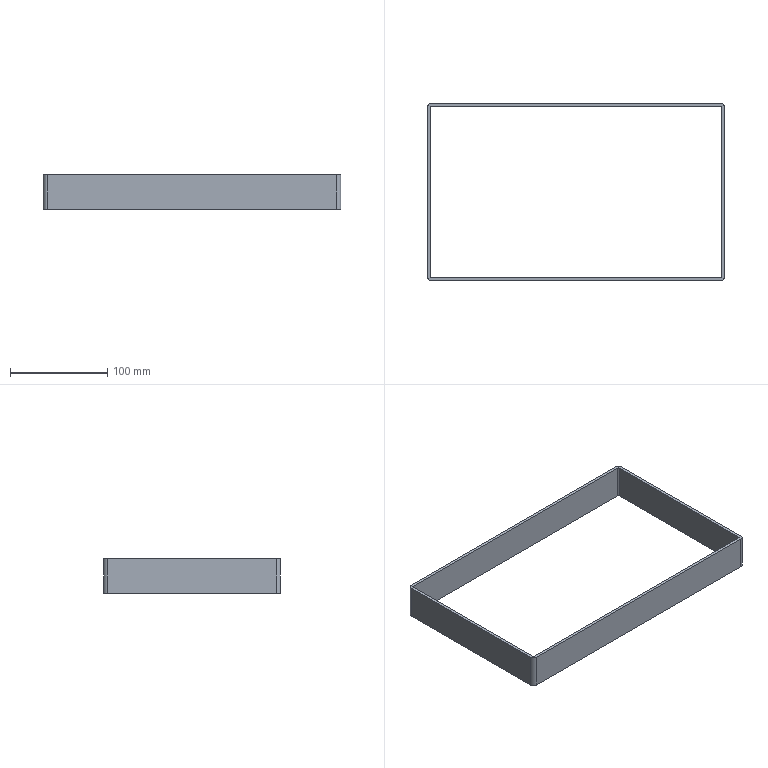Part | NX | features DATUM_CSYS 1, EXTRACT_DATUM_PLANE 1, EXTRUDE 1, SKETCH 1 | 1 solid | 18 faces | box 306 x 182 x 35 mm | volume 100769 mm3 | plane 10 | cylinder 8 | commonest cylinder face diameters 2 x4 8 x4
STEP:
#1=CARTESIAN_POINT('',(-150.,87.,0.));
#2=VERTEX_POINT('',#1);
#3=CARTESIAN_POINT('',(-150.,-87.,0.));
#4=VERTEX_POINT('',#3);
#5=CARTESIAN_POINT('',(-150.,87.,0.));
#6=DIRECTION('',(0.,-1.,0.));
#7=VECTOR('',#6,1000.);
#8=LINE('',#5,#7);
#9=EDGE_CURVE('',#2,#4,#8,.T.);
#10=ORIENTED_EDGE('',*,*,#9,.F.);
#11=CARTESIAN_POINT('',(-150.,87.,35.));
#12=VERTEX_POINT('',#11);
#13=CARTESIAN_POINT('',(-150.,87.,35.));
#14=DIRECTION('',(0.,0.,-1.));
#15=VECTOR('',#14,1000.);
#16=LINE('',#13,#15);
#17=EDGE_CURVE('',#12,#2,#16,.T.);
#18=ORIENTED_EDGE('',*,*,#17,.F.);
#19=CARTESIAN_POINT('',(-150.,-87.,35.));
#20=VERTEX_POINT('',#19);
#21=CARTESIAN_POINT('',(-150.,87.,35.));
#22=DIRECTION('',(0.,-1.,0.));
#23=VECTOR('',#22,1000.);
#24=LINE('',#21,#23);
#25=EDGE_CURVE('',#12,#20,#24,.T.);
#26=ORIENTED_EDGE('',*,*,#25,.T.);
#27=CARTESIAN_POINT('',(-150.,-87.,35.));
#28=DIRECTION('',(0.,0.,-1.));
#29=VECTOR('',#28,1000.);
#30=LINE('',#27,#29);
#31=EDGE_CURVE('',#20,#4,#30,.T.);
#32=ORIENTED_EDGE('',*,*,#31,.T.);
#33=EDGE_LOOP('',(#10,#18,#26,#32));
#34=FACE_BOUND('',#33,.T.);
#35=CARTESIAN_POINT('',(-150.,87.,35.));
#36=DIRECTION('',(1.,0.,0.));
#37=DIRECTION('',(0.,0.,-1.));
#38=AXIS2_PLACEMENT_3D('',#35,#36,#37);
#39=PLANE('',#38);
#40=ADVANCED_FACE('',(#34),#39,.T.);
#41=CARTESIAN_POINT('',(-149.,-88.,0.));
#42=VERTEX_POINT('',#41);
#43=CARTESIAN_POINT('',(-149.,-87.,0.));
#44=DIRECTION('',(0.,0.,1.));
#45=DIRECTION('',(-1.,0.,0.));
#46=AXIS2_PLACEMENT_3D('',#43,#44,#45);
#47=CIRCLE('',#46,1.);
#48=EDGE_CURVE('',#4,#42,#47,.T.);
#49=ORIENTED_EDGE('',*,*,#48,.F.);
#50=ORIENTED_EDGE('',*,*,#31,.F.);
#51=CARTESIAN_POINT('',(-149.,-88.,35.));
#52=VERTEX_POINT('',#51);
#53=CARTESIAN_POINT('',(-149.,-87.,35.));
#54=DIRECTION('',(0.,0.,1.));
#55=DIRECTION('',(-1.,0.,0.));
#56=AXIS2_PLACEMENT_3D('',#53,#54,#55);
#57=CIRCLE('',#56,1.);
#58=EDGE_CURVE('',#20,#52,#57,.T.);
#59=ORIENTED_EDGE('',*,*,#58,.T.);
#60=CARTESIAN_POINT('',(-149.,-88.,35.));
#61=DIRECTION('',(0.,0.,-1.));
#62=VECTOR('',#61,1000.);
#63=LINE('',#60,#62);
#64=EDGE_CURVE('',#52,#42,#63,.T.);
#65=ORIENTED_EDGE('',*,*,#64,.T.);
#66=EDGE_LOOP('',(#49,#50,#59,#65));
#67=FACE_BOUND('',#66,.T.);
#68=CARTESIAN_POINT('',(-149.,-87.,35.));
#69=DIRECTION('',(0.,0.,-1.));
#70=DIRECTION('',(-1.,0.,0.));
#71=AXIS2_PLACEMENT_3D('',#68,#69,#70);
#72=CYLINDRICAL_SURFACE('',#71,1.);
#73=ADVANCED_FACE('',(#67),#72,.F.);
#74=CARTESIAN_POINT('',(149.,-88.,0.));
#75=VERTEX_POINT('',#74);
#76=CARTESIAN_POINT('',(-149.,-88.,0.));
#77=DIRECTION('',(1.,0.,0.));
#78=VECTOR('',#77,1000.);
#79=LINE('',#76,#78);
#80=EDGE_CURVE('',#42,#75,#79,.T.);
#81=ORIENTED_EDGE('',*,*,#80,.F.);
#82=ORIENTED_EDGE('',*,*,#64,.F.);
#83=CARTESIAN_POINT('',(149.,-88.,35.));
#84=VERTEX_POINT('',#83);
#85=CARTESIAN_POINT('',(-149.,-88.,35.));
#86=DIRECTION('',(1.,0.,0.));
#87=VECTOR('',#86,1000.);
#88=LINE('',#85,#87);
#89=EDGE_CURVE('',#52,#84,#88,.T.);
#90=ORIENTED_EDGE('',*,*,#89,.T.);
#91=CARTESIAN_POINT('',(149.,-88.,35.));
#92=DIRECTION('',(0.,0.,-1.));
#93=VECTOR('',#92,1000.);
#94=LINE('',#91,#93);
#95=EDGE_CURVE('',#84,#75,#94,.T.);
#96=ORIENTED_EDGE('',*,*,#95,.T.);
#97=EDGE_LOOP('',(#81,#82,#90,#96));
#98=FACE_BOUND('',#97,.T.);
#99=CARTESIAN_POINT('',(-149.,-88.,35.));
#100=DIRECTION('',(0.,1.,0.));
#101=DIRECTION('',(0.,0.,1.));
#102=AXIS2_PLACEMENT_3D('',#99,#100,#101);
#103=PLANE('',#102);
#104=ADVANCED_FACE('',(#98),#103,.T.);
#105=CARTESIAN_POINT('',(150.,-87.,0.));
#106=VERTEX_POINT('',#105);
#107=CARTESIAN_POINT('',(149.,-87.,0.));
#108=DIRECTION('',(0.,0.,1.));
#109=DIRECTION('',(0.,-1.,0.));
#110=AXIS2_PLACEMENT_3D('',#107,#108,#109);
#111=CIRCLE('',#110,1.);
#112=EDGE_CURVE('',#75,#106,#111,.T.);
#113=ORIENTED_EDGE('',*,*,#112,.F.);
#114=ORIENTED_EDGE('',*,*,#95,.F.);
#115=CARTESIAN_POINT('',(150.,-87.,35.));
#116=VERTEX_POINT('',#115);
#117=CARTESIAN_POINT('',(149.,-87.,35.));
#118=DIRECTION('',(0.,0.,1.));
#119=DIRECTION('',(0.,-1.,0.));
#120=AXIS2_PLACEMENT_3D('',#117,#118,#119);
#121=CIRCLE('',#120,1.);
#122=EDGE_CURVE('',#84,#116,#121,.T.);
#123=ORIENTED_EDGE('',*,*,#122,.T.);
#124=CARTESIAN_POINT('',(150.,-87.,35.));
#125=DIRECTION('',(0.,0.,-1.));
#126=VECTOR('',#125,1000.);
#127=LINE('',#124,#126);
#128=EDGE_CURVE('',#116,#106,#127,.T.);
#129=ORIENTED_EDGE('',*,*,#128,.T.);
#130=EDGE_LOOP('',(#113,#114,#123,#129));
#131=FACE_BOUND('',#130,.T.);
#132=CARTESIAN_POINT('',(149.,-87.,35.));
#133=DIRECTION('',(0.,0.,-1.));
#134=DIRECTION('',(-1.,0.,0.));
#135=AXIS2_PLACEMENT_3D('',#132,#133,#134);
#136=CYLINDRICAL_SURFACE('',#135,1.);
#137=ADVANCED_FACE('',(#131),#136,.F.);
#138=CARTESIAN_POINT('',(150.,87.,0.));
#139=VERTEX_POINT('',#138);
#140=CARTESIAN_POINT('',(150.,-87.,0.));
#141=DIRECTION('',(0.,1.,0.));
#142=VECTOR('',#141,1000.);
#143=LINE('',#140,#142);
#144=EDGE_CURVE('',#106,#139,#143,.T.);
#145=ORIENTED_EDGE('',*,*,#144,.F.);
#146=ORIENTED_EDGE('',*,*,#128,.F.);
#147=CARTESIAN_POINT('',(150.,87.,35.));
#148=VERTEX_POINT('',#147);
#149=CARTESIAN_POINT('',(150.,-87.,35.));
#150=DIRECTION('',(0.,1.,0.));
#151=VECTOR('',#150,1000.);
#152=LINE('',#149,#151);
#153=EDGE_CURVE('',#116,#148,#152,.T.);
#154=ORIENTED_EDGE('',*,*,#153,.T.);
#155=CARTESIAN_POINT('',(150.,87.,35.));
#156=DIRECTION('',(0.,0.,-1.));
#157=VECTOR('',#156,1000.);
#158=LINE('',#155,#157);
#159=EDGE_CURVE('',#148,#139,#158,.T.);
#160=ORIENTED_EDGE('',*,*,#159,.T.);
#161=EDGE_LOOP('',(#145,#146,#154,#160));
#162=FACE_BOUND('',#161,.T.);
#163=CARTESIAN_POINT('',(150.,-87.,35.));
#164=DIRECTION('',(-1.,0.,0.));
#165=DIRECTION('',(0.,0.,1.));
#166=AXIS2_PLACEMENT_3D('',#163,#164,#165);
#167=PLANE('',#166);
#168=ADVANCED_FACE('',(#162),#167,.T.);
#169=CARTESIAN_POINT('',(149.,88.,0.));
#170=VERTEX_POINT('',#169);
#171=CARTESIAN_POINT('',(149.,87.,0.));
#172=DIRECTION('',(0.,0.,1.));
#173=DIRECTION('',(1.,0.,0.));
#174=AXIS2_PLACEMENT_3D('',#171,#172,#173);
#175=CIRCLE('',#174,1.);
#176=EDGE_CURVE('',#139,#170,#175,.T.);
#177=ORIENTED_EDGE('',*,*,#176,.F.);
#178=ORIENTED_EDGE('',*,*,#159,.F.);
#179=CARTESIAN_POINT('',(149.,88.,35.));
#180=VERTEX_POINT('',#179);
#181=CARTESIAN_POINT('',(149.,87.,35.));
#182=DIRECTION('',(0.,0.,1.));
#183=DIRECTION('',(1.,0.,0.));
#184=AXIS2_PLACEMENT_3D('',#181,#182,#183);
#185=CIRCLE('',#184,1.);
#186=EDGE_CURVE('',#148,#180,#185,.T.);
#187=ORIENTED_EDGE('',*,*,#186,.T.);
#188=CARTESIAN_POINT('',(149.,88.,35.));
#189=DIRECTION('',(0.,0.,-1.));
#190=VECTOR('',#189,1000.);
#191=LINE('',#188,#190);
#192=EDGE_CURVE('',#180,#170,#191,.T.);
#193=ORIENTED_EDGE('',*,*,#192,.T.);
#194=EDGE_LOOP('',(#177,#178,#187,#193));
#195=FACE_BOUND('',#194,.T.);
#196=CARTESIAN_POINT('',(149.,87.,35.));
#197=DIRECTION('',(0.,0.,-1.));
#198=DIRECTION('',(-1.,0.,0.));
#199=AXIS2_PLACEMENT_3D('',#196,#197,#198);
#200=CYLINDRICAL_SURFACE('',#199,1.);
#201=ADVANCED_FACE('',(#195),#200,.F.);
#202=CARTESIAN_POINT('',(-149.,88.,0.));
#203=VERTEX_POINT('',#202);
#204=CARTESIAN_POINT('',(149.,88.,0.));
#205=DIRECTION('',(-1.,0.,0.));
#206=VECTOR('',#205,1000.);
#207=LINE('',#204,#206);
#208=EDGE_CURVE('',#170,#203,#207,.T.);
#209=ORIENTED_EDGE('',*,*,#208,.F.);
#210=ORIENTED_EDGE('',*,*,#192,.F.);
#211=CARTESIAN_POINT('',(-149.,88.,35.));
#212=VERTEX_POINT('',#211);
#213=CARTESIAN_POINT('',(149.,88.,35.));
#214=DIRECTION('',(-1.,0.,0.));
#215=VECTOR('',#214,1000.);
#216=LINE('',#213,#215);
#217=EDGE_CURVE('',#180,#212,#216,.T.);
#218=ORIENTED_EDGE('',*,*,#217,.T.);
#219=CARTESIAN_POINT('',(-149.,88.,35.));
#220=DIRECTION('',(0.,0.,-1.));
#221=VECTOR('',#220,1000.);
#222=LINE('',#219,#221);
#223=EDGE_CURVE('',#212,#203,#222,.T.);
#224=ORIENTED_EDGE('',*,*,#223,.T.);
#225=EDGE_LOOP('',(#209,#210,#218,#224));
#226=FACE_BOUND('',#225,.T.);
#227=CARTESIAN_POINT('',(149.,88.,35.));
#228=DIRECTION('',(0.,-1.,0.));
#229=DIRECTION('',(0.,0.,-1.));
#230=AXIS2_PLACEMENT_3D('',#227,#228,#229);
#231=PLANE('',#230);
#232=ADVANCED_FACE('',(#226),#231,.T.);
#233=CARTESIAN_POINT('',(-153.,-87.,0.));
#234=VERTEX_POINT('',#233);
#235=CARTESIAN_POINT('',(-153.,87.,0.));
#236=VERTEX_POINT('',#235);
#237=CARTESIAN_POINT('',(-153.,-87.,0.));
#238=DIRECTION('',(0.,1.,0.));
#239=VECTOR('',#238,1000.);
#240=LINE('',#237,#239);
#241=EDGE_CURVE('',#234,#236,#240,.T.);
#242=ORIENTED_EDGE('',*,*,#241,.F.);
#243=CARTESIAN_POINT('',(-153.,-87.,35.));
#244=VERTEX_POINT('',#243);
#245=CARTESIAN_POINT('',(-153.,-87.,35.));
#246=DIRECTION('',(0.,0.,-1.));
#247=VECTOR('',#246,1000.);
#248=LINE('',#245,#247);
#249=EDGE_CURVE('',#244,#234,#248,.T.);
#250=ORIENTED_EDGE('',*,*,#249,.F.);
#251=CARTESIAN_POINT('',(-153.,87.,35.));
#252=VERTEX_POINT('',#251);
#253=CARTESIAN_POINT('',(-153.,-87.,35.));
#254=DIRECTION('',(0.,1.,0.));
#255=VECTOR('',#254,1000.);
#256=LINE('',#253,#255);
#257=EDGE_CURVE('',#244,#252,#256,.T.);
#258=ORIENTED_EDGE('',*,*,#257,.T.);
#259=CARTESIAN_POINT('',(-153.,87.,35.));
#260=DIRECTION('',(0.,0.,-1.));
#261=VECTOR('',#260,1000.);
#262=LINE('',#259,#261);
#263=EDGE_CURVE('',#252,#236,#262,.T.);
#264=ORIENTED_EDGE('',*,*,#263,.T.);
#265=EDGE_LOOP('',(#242,#250,#258,#264));
#266=FACE_BOUND('',#265,.T.);
#267=CARTESIAN_POINT('',(-153.,-87.,35.));
#268=DIRECTION('',(-1.,0.,0.));
#269=DIRECTION('',(0.,0.,1.));
#270=AXIS2_PLACEMENT_3D('',#267,#268,#269);
#271=PLANE('',#270);
#272=ADVANCED_FACE('',(#266),#271,.T.);
#273=CARTESIAN_POINT('',(-149.,91.,0.));
#274=VERTEX_POINT('',#273);
#275=CARTESIAN_POINT('',(-149.,87.,0.));
#276=DIRECTION('',(0.,0.,-1.));
#277=DIRECTION('',(-1.,0.,0.));
#278=AXIS2_PLACEMENT_3D('',#275,#276,#277);
#279=CIRCLE('',#278,4.);
#280=EDGE_CURVE('',#236,#274,#279,.T.);
#281=ORIENTED_EDGE('',*,*,#280,.F.);
#282=ORIENTED_EDGE('',*,*,#263,.F.);
#283=CARTESIAN_POINT('',(-149.,91.,35.));
#284=VERTEX_POINT('',#283);
#285=CARTESIAN_POINT('',(-149.,87.,35.));
#286=DIRECTION('',(0.,0.,-1.));
#287=DIRECTION('',(-1.,0.,0.));
#288=AXIS2_PLACEMENT_3D('',#285,#286,#287);
#289=CIRCLE('',#288,4.);
#290=EDGE_CURVE('',#252,#284,#289,.T.);
#291=ORIENTED_EDGE('',*,*,#290,.T.);
#292=CARTESIAN_POINT('',(-149.,91.,35.));
#293=DIRECTION('',(0.,0.,-1.));
#294=VECTOR('',#293,1000.);
#295=LINE('',#292,#294);
#296=EDGE_CURVE('',#284,#274,#295,.T.);
#297=ORIENTED_EDGE('',*,*,#296,.T.);
#298=EDGE_LOOP('',(#281,#282,#291,#297));
#299=FACE_BOUND('',#298,.T.);
#300=CARTESIAN_POINT('',(-149.,87.,35.));
#301=DIRECTION('',(0.,0.,-1.));
#302=DIRECTION('',(-1.,0.,0.));
#303=AXIS2_PLACEMENT_3D('',#300,#301,#302);
#304=CYLINDRICAL_SURFACE('',#303,4.);
#305=ADVANCED_FACE('',(#299),#304,.T.);
#306=CARTESIAN_POINT('',(149.,91.,0.));
#307=VERTEX_POINT('',#306);
#308=CARTESIAN_POINT('',(-149.,91.,0.));
#309=DIRECTION('',(1.,0.,0.));
#310=VECTOR('',#309,1000.);
#311=LINE('',#308,#310);
#312=EDGE_CURVE('',#274,#307,#311,.T.);
#313=ORIENTED_EDGE('',*,*,#312,.F.);
#314=ORIENTED_EDGE('',*,*,#296,.F.);
#315=CARTESIAN_POINT('',(149.,91.,35.));
#316=VERTEX_POINT('',#315);
#317=CARTESIAN_POINT('',(-149.,91.,35.));
#318=DIRECTION('',(1.,0.,0.));
#319=VECTOR('',#318,1000.);
#320=LINE('',#317,#319);
#321=EDGE_CURVE('',#284,#316,#320,.T.);
#322=ORIENTED_EDGE('',*,*,#321,.T.);
#323=CARTESIAN_POINT('',(149.,91.,35.));
#324=DIRECTION('',(0.,0.,-1.));
#325=VECTOR('',#324,1000.);
#326=LINE('',#323,#325);
#327=EDGE_CURVE('',#316,#307,#326,.T.);
#328=ORIENTED_EDGE('',*,*,#327,.T.);
#329=EDGE_LOOP('',(#313,#314,#322,#328));
#330=FACE_BOUND('',#329,.T.);
#331=CARTESIAN_POINT('',(-149.,91.,35.));
#332=DIRECTION('',(0.,1.,0.));
#333=DIRECTION('',(0.,0.,1.));
#334=AXIS2_PLACEMENT_3D('',#331,#332,#333);
#335=PLANE('',#334);
#336=ADVANCED_FACE('',(#330),#335,.T.);
#337=CARTESIAN_POINT('',(153.,87.,0.));
#338=VERTEX_POINT('',#337);
#339=CARTESIAN_POINT('',(149.,87.,0.));
#340=DIRECTION('',(0.,0.,-1.));
#341=DIRECTION('',(0.,1.,0.));
#342=AXIS2_PLACEMENT_3D('',#339,#340,#341);
#343=CIRCLE('',#342,4.);
#344=EDGE_CURVE('',#307,#338,#343,.T.);
#345=ORIENTED_EDGE('',*,*,#344,.F.);
#346=ORIENTED_EDGE('',*,*,#327,.F.);
#347=CARTESIAN_POINT('',(153.,87.,35.));
#348=VERTEX_POINT('',#347);
#349=CARTESIAN_POINT('',(149.,87.,35.));
#350=DIRECTION('',(0.,0.,-1.));
#351=DIRECTION('',(0.,1.,0.));
#352=AXIS2_PLACEMENT_3D('',#349,#350,#351);
#353=CIRCLE('',#352,4.);
#354=EDGE_CURVE('',#316,#348,#353,.T.);
#355=ORIENTED_EDGE('',*,*,#354,.T.);
#356=CARTESIAN_POINT('',(153.,87.,35.));
#357=DIRECTION('',(0.,0.,-1.));
#358=VECTOR('',#357,1000.);
#359=LINE('',#356,#358);
#360=EDGE_CURVE('',#348,#338,#359,.T.);
#361=ORIENTED_EDGE('',*,*,#360,.T.);
#362=EDGE_LOOP('',(#345,#346,#355,#361));
#363=FACE_BOUND('',#362,.T.);
#364=CARTESIAN_POINT('',(149.,87.,35.));
#365=DIRECTION('',(0.,0.,-1.));
#366=DIRECTION('',(-1.,0.,0.));
#367=AXIS2_PLACEMENT_3D('',#364,#365,#366);
#368=CYLINDRICAL_SURFACE('',#367,4.);
#369=ADVANCED_FACE('',(#363),#368,.T.);
#370=CARTESIAN_POINT('',(153.,-87.,0.));
#371=VERTEX_POINT('',#370);
#372=CARTESIAN_POINT('',(153.,87.,0.));
#373=DIRECTION('',(0.,-1.,0.));
#374=VECTOR('',#373,1000.);
#375=LINE('',#372,#374);
#376=EDGE_CURVE('',#338,#371,#375,.T.);
#377=ORIENTED_EDGE('',*,*,#376,.F.);
#378=ORIENTED_EDGE('',*,*,#360,.F.);
#379=CARTESIAN_POINT('',(153.,-87.,35.));
#380=VERTEX_POINT('',#379);
#381=CARTESIAN_POINT('',(153.,87.,35.));
#382=DIRECTION('',(0.,-1.,0.));
#383=VECTOR('',#382,1000.);
#384=LINE('',#381,#383);
#385=EDGE_CURVE('',#348,#380,#384,.T.);
#386=ORIENTED_EDGE('',*,*,#385,.T.);
#387=CARTESIAN_POINT('',(153.,-87.,35.));
#388=DIRECTION('',(0.,0.,-1.));
#389=VECTOR('',#388,1000.);
#390=LINE('',#387,#389);
#391=EDGE_CURVE('',#380,#371,#390,.T.);
#392=ORIENTED_EDGE('',*,*,#391,.T.);
#393=EDGE_LOOP('',(#377,#378,#386,#392));
#394=FACE_BOUND('',#393,.T.);
#395=CARTESIAN_POINT('',(153.,87.,35.));
#396=DIRECTION('',(1.,0.,0.));
#397=DIRECTION('',(0.,0.,-1.));
#398=AXIS2_PLACEMENT_3D('',#395,#396,#397);
#399=PLANE('',#398);
#400=ADVANCED_FACE('',(#394),#399,.T.);
#401=CARTESIAN_POINT('',(149.,-91.,0.));
#402=VERTEX_POINT('',#401);
#403=CARTESIAN_POINT('',(149.,-87.,0.));
#404=DIRECTION('',(0.,0.,-1.));
#405=DIRECTION('',(1.,0.,0.));
#406=AXIS2_PLACEMENT_3D('',#403,#404,#405);
#407=CIRCLE('',#406,4.);
#408=EDGE_CURVE('',#371,#402,#407,.T.);
#409=ORIENTED_EDGE('',*,*,#408,.F.);
#410=ORIENTED_EDGE('',*,*,#391,.F.);
#411=CARTESIAN_POINT('',(149.,-91.,35.));
#412=VERTEX_POINT('',#411);
#413=CARTESIAN_POINT('',(149.,-87.,35.));
#414=DIRECTION('',(0.,0.,-1.));
#415=DIRECTION('',(1.,0.,0.));
#416=AXIS2_PLACEMENT_3D('',#413,#414,#415);
#417=CIRCLE('',#416,4.);
#418=EDGE_CURVE('',#380,#412,#417,.T.);
#419=ORIENTED_EDGE('',*,*,#418,.T.);
#420=CARTESIAN_POINT('',(149.,-91.,35.));
#421=DIRECTION('',(0.,0.,-1.));
#422=VECTOR('',#421,1000.);
#423=LINE('',#420,#422);
#424=EDGE_CURVE('',#412,#402,#423,.T.);
#425=ORIENTED_EDGE('',*,*,#424,.T.);
#426=EDGE_LOOP('',(#409,#410,#419,#425));
#427=FACE_BOUND('',#426,.T.);
#428=CARTESIAN_POINT('',(149.,-87.,35.));
#429=DIRECTION('',(0.,0.,-1.));
#430=DIRECTION('',(-1.,0.,0.));
#431=AXIS2_PLACEMENT_3D('',#428,#429,#430);
#432=CYLINDRICAL_SURFACE('',#431,4.);
#433=ADVANCED_FACE('',(#427),#432,.T.);
#434=CARTESIAN_POINT('',(-149.,-91.,0.));
#435=VERTEX_POINT('',#434);
#436=CARTESIAN_POINT('',(149.,-91.,0.));
#437=DIRECTION('',(-1.,0.,0.));
#438=VECTOR('',#437,1000.);
#439=LINE('',#436,#438);
#440=EDGE_CURVE('',#402,#435,#439,.T.);
#441=ORIENTED_EDGE('',*,*,#440,.F.);
#442=ORIENTED_EDGE('',*,*,#424,.F.);
#443=CARTESIAN_POINT('',(-149.,-91.,35.));
#444=VERTEX_POINT('',#443);
#445=CARTESIAN_POINT('',(149.,-91.,35.));
#446=DIRECTION('',(-1.,0.,0.));
#447=VECTOR('',#446,1000.);
#448=LINE('',#445,#447);
#449=EDGE_CURVE('',#412,#444,#448,.T.);
#450=ORIENTED_EDGE('',*,*,#449,.T.);
#451=CARTESIAN_POINT('',(-149.,-91.,35.));
#452=DIRECTION('',(0.,0.,-1.));
#453=VECTOR('',#452,1000.);
#454=LINE('',#451,#453);
#455=EDGE_CURVE('',#444,#435,#454,.T.);
#456=ORIENTED_EDGE('',*,*,#455,.T.);
#457=EDGE_LOOP('',(#441,#442,#450,#456));
#458=FACE_BOUND('',#457,.T.);
#459=CARTESIAN_POINT('',(149.,-91.,35.));
#460=DIRECTION('',(0.,-1.,0.));
#461=DIRECTION('',(0.,0.,-1.));
#462=AXIS2_PLACEMENT_3D('',#459,#460,#461);
#463=PLANE('',#462);
#464=ADVANCED_FACE('',(#458),#463,.T.);
#465=CARTESIAN_POINT('',(-149.,-87.,0.));
#466=DIRECTION('',(0.,0.,-1.));
#467=DIRECTION('',(0.,-1.,0.));
#468=AXIS2_PLACEMENT_3D('',#465,#466,#467);
#469=CIRCLE('',#468,4.);
#470=EDGE_CURVE('',#435,#234,#469,.T.);
#471=ORIENTED_EDGE('',*,*,#470,.F.);
#472=ORIENTED_EDGE('',*,*,#455,.F.);
#473=CARTESIAN_POINT('',(-149.,-87.,35.));
#474=DIRECTION('',(0.,0.,-1.));
#475=DIRECTION('',(0.,-1.,0.));
#476=AXIS2_PLACEMENT_3D('',#473,#474,#475);
#477=CIRCLE('',#476,4.);
#478=EDGE_CURVE('',#444,#244,#477,.T.);
#479=ORIENTED_EDGE('',*,*,#478,.T.);
#480=ORIENTED_EDGE('',*,*,#249,.T.);
#481=EDGE_LOOP('',(#471,#472,#479,#480));
#482=FACE_BOUND('',#481,.T.);
#483=CARTESIAN_POINT('',(-149.,-87.,35.));
#484=DIRECTION('',(0.,0.,-1.));
#485=DIRECTION('',(-1.,0.,0.));
#486=AXIS2_PLACEMENT_3D('',#483,#484,#485);
#487=CYLINDRICAL_SURFACE('',#486,4.);
#488=ADVANCED_FACE('',(#482),#487,.T.);
#489=CARTESIAN_POINT('',(-149.,87.,0.));
#490=DIRECTION('',(0.,0.,1.));
#491=DIRECTION('',(0.,1.,0.));
#492=AXIS2_PLACEMENT_3D('',#489,#490,#491);
#493=CIRCLE('',#492,1.);
#494=EDGE_CURVE('',#203,#2,#493,.T.);
#495=ORIENTED_EDGE('',*,*,#494,.F.);
#496=ORIENTED_EDGE('',*,*,#223,.F.);
#497=CARTESIAN_POINT('',(-149.,87.,35.));
#498=DIRECTION('',(0.,0.,1.));
#499=DIRECTION('',(0.,1.,0.));
#500=AXIS2_PLACEMENT_3D('',#497,#498,#499);
#501=CIRCLE('',#500,1.);
#502=EDGE_CURVE('',#212,#12,#501,.T.);
#503=ORIENTED_EDGE('',*,*,#502,.T.);
#504=ORIENTED_EDGE('',*,*,#17,.T.);
#505=EDGE_LOOP('',(#495,#496,#503,#504));
#506=FACE_BOUND('',#505,.T.);
#507=CARTESIAN_POINT('',(-149.,87.,35.));
#508=DIRECTION('',(0.,0.,-1.));
#509=DIRECTION('',(-1.,0.,0.));
#510=AXIS2_PLACEMENT_3D('',#507,#508,#509);
#511=CYLINDRICAL_SURFACE('',#510,1.);
#512=ADVANCED_FACE('',(#506),#511,.F.);
#513=ORIENTED_EDGE('',*,*,#257,.F.);
#514=ORIENTED_EDGE('',*,*,#478,.F.);
#515=ORIENTED_EDGE('',*,*,#449,.F.);
#516=ORIENTED_EDGE('',*,*,#418,.F.);
#517=ORIENTED_EDGE('',*,*,#385,.F.);
#518=ORIENTED_EDGE('',*,*,#354,.F.);
#519=ORIENTED_EDGE('',*,*,#321,.F.);
#520=ORIENTED_EDGE('',*,*,#290,.F.);
#521=EDGE_LOOP('',(#513,#514,#515,#516,#517,#518,#519,#520));
#522=FACE_BOUND('',#521,.T.);
#523=ORIENTED_EDGE('',*,*,#25,.F.);
#524=ORIENTED_EDGE('',*,*,#502,.F.);
#525=ORIENTED_EDGE('',*,*,#217,.F.);
#526=ORIENTED_EDGE('',*,*,#186,.F.);
#527=ORIENTED_EDGE('',*,*,#153,.F.);
#528=ORIENTED_EDGE('',*,*,#122,.F.);
#529=ORIENTED_EDGE('',*,*,#89,.F.);
#530=ORIENTED_EDGE('',*,*,#58,.F.);
#531=EDGE_LOOP('',(#523,#524,#525,#526,#527,#528,#529,#530));
#532=FACE_BOUND('',#531,.T.);
#533=CARTESIAN_POINT('',(-149.,87.,35.));
#534=DIRECTION('',(0.,0.,-1.));
#535=DIRECTION('',(-1.,0.,0.));
#536=AXIS2_PLACEMENT_3D('',#533,#534,#535);
#537=PLANE('',#536);
#538=ADVANCED_FACE('',(#522,#532),#537,.F.);
#539=ORIENTED_EDGE('',*,*,#241,.T.);
#540=ORIENTED_EDGE('',*,*,#280,.T.);
#541=ORIENTED_EDGE('',*,*,#312,.T.);
#542=ORIENTED_EDGE('',*,*,#344,.T.);
#543=ORIENTED_EDGE('',*,*,#376,.T.);
#544=ORIENTED_EDGE('',*,*,#408,.T.);
#545=ORIENTED_EDGE('',*,*,#440,.T.);
#546=ORIENTED_EDGE('',*,*,#470,.T.);
#547=EDGE_LOOP('',(#539,#540,#541,#542,#543,#544,#545,#546));
#548=FACE_BOUND('',#547,.T.);
#549=ORIENTED_EDGE('',*,*,#9,.T.);
#550=ORIENTED_EDGE('',*,*,#48,.T.);
#551=ORIENTED_EDGE('',*,*,#80,.T.);
#552=ORIENTED_EDGE('',*,*,#112,.T.);
#553=ORIENTED_EDGE('',*,*,#144,.T.);
#554=ORIENTED_EDGE('',*,*,#176,.T.);
#555=ORIENTED_EDGE('',*,*,#208,.T.);
#556=ORIENTED_EDGE('',*,*,#494,.T.);
#557=EDGE_LOOP('',(#549,#550,#551,#552,#553,#554,#555,#556));
#558=FACE_BOUND('',#557,.T.);
#559=CARTESIAN_POINT('',(-149.,87.,0.));
#560=DIRECTION('',(0.,0.,-1.));
#561=DIRECTION('',(-1.,0.,0.));
#562=AXIS2_PLACEMENT_3D('',#559,#560,#561);
#563=PLANE('',#562);
#564=ADVANCED_FACE('',(#548,#558),#563,.T.);
#565=CLOSED_SHELL('',(#40,#73,#104,#137,#168,#201,#232,#272,#305,#336,#369,#400,#433,#464,#488,#512,#538,#564));
#566=MANIFOLD_SOLID_BREP('',#565);
#567=(LENGTH_UNIT()NAMED_UNIT(*)SI_UNIT(.MILLI.,.METRE.));
#568=UNCERTAINTY_MEASURE_WITH_UNIT(LENGTH_MEASURE(0.00001),#567,'','');
#569=(NAMED_UNIT(*)PLANE_ANGLE_UNIT()SI_UNIT($,.RADIAN.));
#570=(NAMED_UNIT(*)SI_UNIT($,.STERADIAN.)SOLID_ANGLE_UNIT());
#571=(GEOMETRIC_REPRESENTATION_CONTEXT(3)GLOBAL_UNCERTAINTY_ASSIGNED_CONTEXT((#568))GLOBAL_UNIT_ASSIGNED_CONTEXT((#567,#569,#570))REPRESENTATION_CONTEXT('',''));
#572=ADVANCED_BREP_SHAPE_REPRESENTATION('',(#566),#571);